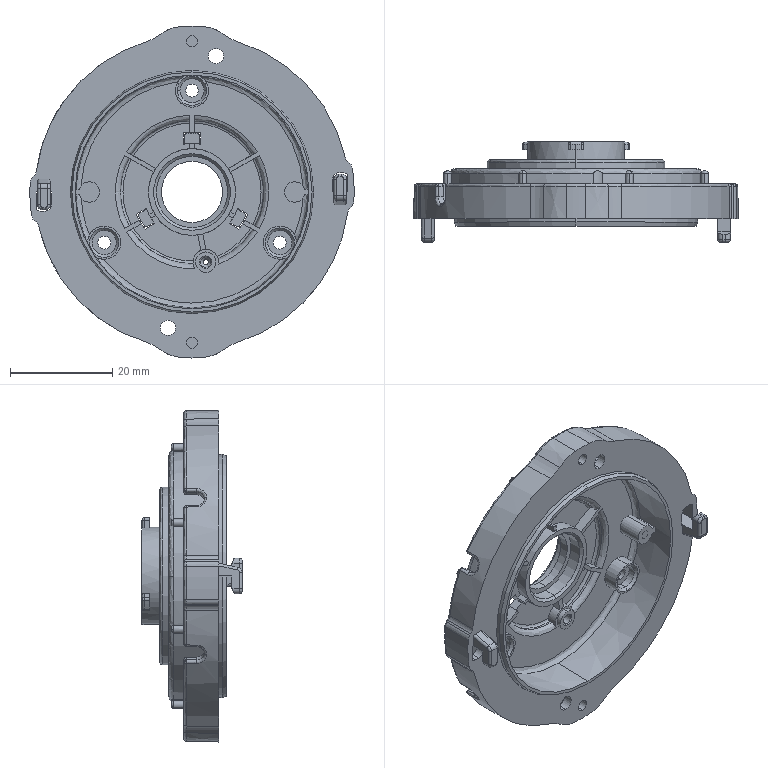Part | SolidWorks | features BaseBody 1 | 1 solid | 486 faces | box 63.5 x 19.6 x 65 mm | volume 11107 mm3 | plane 158 | cylinder 137 | spline 126 | cone 64 | torus 1 | commonest cylinder face diameters 1 x28 1.5 x16 2.5 x10 5 x10 3 x8 4 x8